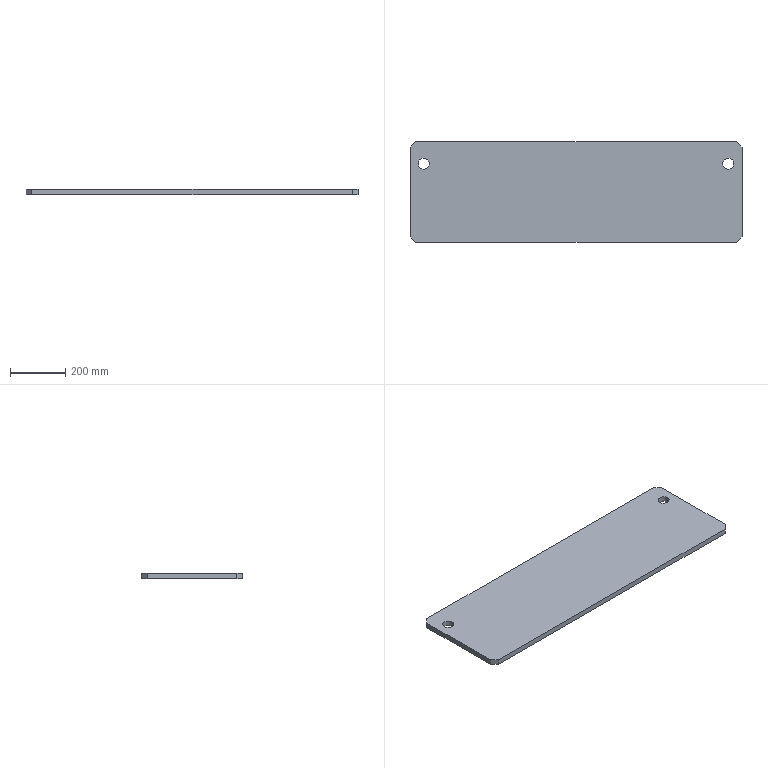Part | SolidWorks | features Chamfer 2, Extrusion 1, ICE 1 | 1 solid | 14 faces | box 1200 x 365 x 20 mm | volume 8693735 mm3 | plane 10 | cylinder 4 | commonest cylinder face diameters 40 x4
STEP:
#1=CARTESIAN_POINT('',(-570.,102.5,0.));
#2=VERTEX_POINT('',#1);
#3=CARTESIAN_POINT('',(-530.,102.5,0.));
#4=VERTEX_POINT('',#3);
#5=CARTESIAN_POINT('',(-550.,102.5,0.));
#6=DIRECTION('',(0.,0.,1.));
#7=DIRECTION('',(1.,0.,0.));
#8=AXIS2_PLACEMENT_3D('',#5,#6,#7);
#9=CIRCLE('',#8,20.);
#10=EDGE_CURVE('',#2,#4,#9,.T.);
#11=ORIENTED_EDGE('',*,*,#10,.F.);
#12=CARTESIAN_POINT('',(-570.,102.5,20.));
#13=VERTEX_POINT('',#12);
#14=CARTESIAN_POINT('',(-570.,102.5,0.));
#15=DIRECTION('',(0.,0.,1.));
#16=VECTOR('',#15,1000.);
#17=LINE('',#14,#16);
#18=EDGE_CURVE('',#2,#13,#17,.T.);
#19=ORIENTED_EDGE('',*,*,#18,.T.);
#20=CARTESIAN_POINT('',(-530.,102.5,20.));
#21=VERTEX_POINT('',#20);
#22=CARTESIAN_POINT('',(-550.,102.5,20.));
#23=DIRECTION('',(0.,0.,1.));
#24=DIRECTION('',(1.,0.,0.));
#25=AXIS2_PLACEMENT_3D('',#22,#23,#24);
#26=CIRCLE('',#25,20.);
#27=EDGE_CURVE('',#13,#21,#26,.T.);
#28=ORIENTED_EDGE('',*,*,#27,.T.);
#29=CARTESIAN_POINT('',(-530.,102.5,0.));
#30=DIRECTION('',(0.,0.,1.));
#31=VECTOR('',#30,1000.);
#32=LINE('',#29,#31);
#33=EDGE_CURVE('',#4,#21,#32,.T.);
#34=ORIENTED_EDGE('',*,*,#33,.F.);
#35=EDGE_LOOP('',(#11,#19,#28,#34));
#36=FACE_OUTER_BOUND('',#35,.T.);
#37=CARTESIAN_POINT('',(-550.,102.5,0.));
#38=DIRECTION('',(0.,0.,1.));
#39=DIRECTION('',(1.,0.,0.));
#40=AXIS2_PLACEMENT_3D('',#37,#38,#39);
#41=CYLINDRICAL_SURFACE('',#40,20.);
#42=ADVANCED_FACE('',(#36),#41,.F.);
#43=CARTESIAN_POINT('',(530.,102.5,0.));
#44=VERTEX_POINT('',#43);
#45=CARTESIAN_POINT('',(570.,102.5,0.));
#46=VERTEX_POINT('',#45);
#47=CARTESIAN_POINT('',(550.,102.5,0.));
#48=DIRECTION('',(0.,0.,1.));
#49=DIRECTION('',(-1.,0.,0.));
#50=AXIS2_PLACEMENT_3D('',#47,#48,#49);
#51=CIRCLE('',#50,20.);
#52=EDGE_CURVE('',#44,#46,#51,.T.);
#53=ORIENTED_EDGE('',*,*,#52,.F.);
#54=CARTESIAN_POINT('',(530.,102.5,20.));
#55=VERTEX_POINT('',#54);
#56=CARTESIAN_POINT('',(530.,102.5,0.));
#57=DIRECTION('',(0.,0.,1.));
#58=VECTOR('',#57,1000.);
#59=LINE('',#56,#58);
#60=EDGE_CURVE('',#44,#55,#59,.T.);
#61=ORIENTED_EDGE('',*,*,#60,.T.);
#62=CARTESIAN_POINT('',(570.,102.5,20.));
#63=VERTEX_POINT('',#62);
#64=CARTESIAN_POINT('',(550.,102.5,20.));
#65=DIRECTION('',(0.,0.,1.));
#66=DIRECTION('',(1.,0.,0.));
#67=AXIS2_PLACEMENT_3D('',#64,#65,#66);
#68=CIRCLE('',#67,20.);
#69=EDGE_CURVE('',#55,#63,#68,.T.);
#70=ORIENTED_EDGE('',*,*,#69,.T.);
#71=CARTESIAN_POINT('',(570.,102.5,0.));
#72=DIRECTION('',(0.,0.,1.));
#73=VECTOR('',#72,1000.);
#74=LINE('',#71,#73);
#75=EDGE_CURVE('',#46,#63,#74,.T.);
#76=ORIENTED_EDGE('',*,*,#75,.F.);
#77=EDGE_LOOP('',(#53,#61,#70,#76));
#78=FACE_OUTER_BOUND('',#77,.T.);
#79=CARTESIAN_POINT('',(550.,102.5,0.));
#80=DIRECTION('',(0.,0.,1.));
#81=DIRECTION('',(1.,0.,0.));
#82=AXIS2_PLACEMENT_3D('',#79,#80,#81);
#83=CYLINDRICAL_SURFACE('',#82,20.);
#84=ADVANCED_FACE('',(#78),#83,.F.);
#85=CARTESIAN_POINT('',(600.,-162.5,20.));
#86=VERTEX_POINT('',#85);
#87=CARTESIAN_POINT('',(600.,162.5,20.));
#88=VERTEX_POINT('',#87);
#89=CARTESIAN_POINT('',(600.,182.5,20.));
#90=DIRECTION('',(0.,1.,0.));
#91=VECTOR('',#90,1000.);
#92=LINE('',#89,#91);
#93=EDGE_CURVE('',#86,#88,#92,.T.);
#94=ORIENTED_EDGE('',*,*,#93,.F.);
#95=CARTESIAN_POINT('',(600.,-162.5,0.));
#96=VERTEX_POINT('',#95);
#97=CARTESIAN_POINT('',(600.,-162.5,20.));
#98=DIRECTION('',(0.,0.,-1.));
#99=VECTOR('',#98,1000.);
#100=LINE('',#97,#99);
#101=EDGE_CURVE('',#86,#96,#100,.T.);
#102=ORIENTED_EDGE('',*,*,#101,.T.);
#103=CARTESIAN_POINT('',(600.,162.5,0.));
#104=VERTEX_POINT('',#103);
#105=CARTESIAN_POINT('',(600.,182.5,0.));
#106=DIRECTION('',(0.,1.,0.));
#107=VECTOR('',#106,1000.);
#108=LINE('',#105,#107);
#109=EDGE_CURVE('',#96,#104,#108,.T.);
#110=ORIENTED_EDGE('',*,*,#109,.T.);
#111=CARTESIAN_POINT('',(600.,162.5,20.));
#112=DIRECTION('',(0.,0.,1.));
#113=VECTOR('',#112,1000.);
#114=LINE('',#111,#113);
#115=EDGE_CURVE('',#104,#88,#114,.T.);
#116=ORIENTED_EDGE('',*,*,#115,.T.);
#117=EDGE_LOOP('',(#94,#102,#110,#116));
#118=FACE_OUTER_BOUND('',#117,.T.);
#119=CARTESIAN_POINT('',(600.,182.5,20.));
#120=DIRECTION('',(-1.,0.,0.));
#121=DIRECTION('',(0.,-1.,0.));
#122=AXIS2_PLACEMENT_3D('',#119,#120,#121);
#123=PLANE('',#122);
#124=ADVANCED_FACE('',(#118),#123,.F.);
#125=CARTESIAN_POINT('',(580.,182.5,20.));
#126=VERTEX_POINT('',#125);
#127=CARTESIAN_POINT('',(-580.,182.5,20.));
#128=VERTEX_POINT('',#127);
#129=CARTESIAN_POINT('',(-600.,182.5,20.));
#130=DIRECTION('',(-1.,0.,0.));
#131=VECTOR('',#130,1000.);
#132=LINE('',#129,#131);
#133=EDGE_CURVE('',#126,#128,#132,.T.);
#134=ORIENTED_EDGE('',*,*,#133,.F.);
#135=CARTESIAN_POINT('',(580.,182.5,0.));
#136=VERTEX_POINT('',#135);
#137=CARTESIAN_POINT('',(580.,182.5,20.));
#138=DIRECTION('',(0.,0.,-1.));
#139=VECTOR('',#138,1000.);
#140=LINE('',#137,#139);
#141=EDGE_CURVE('',#126,#136,#140,.T.);
#142=ORIENTED_EDGE('',*,*,#141,.T.);
#143=CARTESIAN_POINT('',(-580.,182.5,0.));
#144=VERTEX_POINT('',#143);
#145=CARTESIAN_POINT('',(-600.,182.5,0.));
#146=DIRECTION('',(-1.,0.,0.));
#147=VECTOR('',#146,1000.);
#148=LINE('',#145,#147);
#149=EDGE_CURVE('',#136,#144,#148,.T.);
#150=ORIENTED_EDGE('',*,*,#149,.T.);
#151=CARTESIAN_POINT('',(-580.,182.5,20.));
#152=DIRECTION('',(0.,0.,1.));
#153=VECTOR('',#152,1000.);
#154=LINE('',#151,#153);
#155=EDGE_CURVE('',#144,#128,#154,.T.);
#156=ORIENTED_EDGE('',*,*,#155,.T.);
#157=EDGE_LOOP('',(#134,#142,#150,#156));
#158=FACE_OUTER_BOUND('',#157,.T.);
#159=CARTESIAN_POINT('',(-600.,182.5,20.));
#160=DIRECTION('',(0.,-1.,0.));
#161=DIRECTION('',(0.,0.,-1.));
#162=AXIS2_PLACEMENT_3D('',#159,#160,#161);
#163=PLANE('',#162);
#164=ADVANCED_FACE('',(#158),#163,.F.);
#165=CARTESIAN_POINT('',(-600.,162.5,0.));
#166=VERTEX_POINT('',#165);
#167=CARTESIAN_POINT('',(-600.,-162.5,0.));
#168=VERTEX_POINT('',#167);
#169=CARTESIAN_POINT('',(-600.,182.5,0.));
#170=DIRECTION('',(0.,-1.,0.));
#171=VECTOR('',#170,1000.);
#172=LINE('',#169,#171);
#173=EDGE_CURVE('',#166,#168,#172,.T.);
#174=ORIENTED_EDGE('',*,*,#173,.T.);
#175=CARTESIAN_POINT('',(-600.,-162.5,20.));
#176=VERTEX_POINT('',#175);
#177=CARTESIAN_POINT('',(-600.,-162.5,20.));
#178=DIRECTION('',(0.,0.,1.));
#179=VECTOR('',#178,1000.);
#180=LINE('',#177,#179);
#181=EDGE_CURVE('',#168,#176,#180,.T.);
#182=ORIENTED_EDGE('',*,*,#181,.T.);
#183=CARTESIAN_POINT('',(-600.,162.5,20.));
#184=VERTEX_POINT('',#183);
#185=CARTESIAN_POINT('',(-600.,182.5,20.));
#186=DIRECTION('',(0.,-1.,0.));
#187=VECTOR('',#186,1000.);
#188=LINE('',#185,#187);
#189=EDGE_CURVE('',#184,#176,#188,.T.);
#190=ORIENTED_EDGE('',*,*,#189,.F.);
#191=CARTESIAN_POINT('',(-600.,162.5,20.));
#192=DIRECTION('',(0.,0.,-1.));
#193=VECTOR('',#192,1000.);
#194=LINE('',#191,#193);
#195=EDGE_CURVE('',#184,#166,#194,.T.);
#196=ORIENTED_EDGE('',*,*,#195,.T.);
#197=EDGE_LOOP('',(#174,#182,#190,#196));
#198=FACE_OUTER_BOUND('',#197,.T.);
#199=CARTESIAN_POINT('',(-600.,182.5,20.));
#200=DIRECTION('',(1.,0.,0.));
#201=DIRECTION('',(0.,1.,0.));
#202=AXIS2_PLACEMENT_3D('',#199,#200,#201);
#203=PLANE('',#202);
#204=ADVANCED_FACE('',(#198),#203,.F.);
#205=CARTESIAN_POINT('',(-580.,-182.5,20.));
#206=VERTEX_POINT('',#205);
#207=CARTESIAN_POINT('',(580.,-182.5,20.));
#208=VERTEX_POINT('',#207);
#209=CARTESIAN_POINT('',(-600.,-182.5,20.));
#210=DIRECTION('',(1.,0.,0.));
#211=VECTOR('',#210,1000.);
#212=LINE('',#209,#211);
#213=EDGE_CURVE('',#206,#208,#212,.T.);
#214=ORIENTED_EDGE('',*,*,#213,.F.);
#215=CARTESIAN_POINT('',(-580.,-182.5,0.));
#216=VERTEX_POINT('',#215);
#217=CARTESIAN_POINT('',(-580.,-182.5,20.));
#218=DIRECTION('',(0.,0.,-1.));
#219=VECTOR('',#218,1000.);
#220=LINE('',#217,#219);
#221=EDGE_CURVE('',#206,#216,#220,.T.);
#222=ORIENTED_EDGE('',*,*,#221,.T.);
#223=CARTESIAN_POINT('',(580.,-182.5,0.));
#224=VERTEX_POINT('',#223);
#225=CARTESIAN_POINT('',(-600.,-182.5,0.));
#226=DIRECTION('',(1.,0.,0.));
#227=VECTOR('',#226,1000.);
#228=LINE('',#225,#227);
#229=EDGE_CURVE('',#216,#224,#228,.T.);
#230=ORIENTED_EDGE('',*,*,#229,.T.);
#231=CARTESIAN_POINT('',(580.,-182.5,20.));
#232=DIRECTION('',(0.,0.,1.));
#233=VECTOR('',#232,1000.);
#234=LINE('',#231,#233);
#235=EDGE_CURVE('',#224,#208,#234,.T.);
#236=ORIENTED_EDGE('',*,*,#235,.T.);
#237=EDGE_LOOP('',(#214,#222,#230,#236));
#238=FACE_OUTER_BOUND('',#237,.T.);
#239=CARTESIAN_POINT('',(-600.,-182.5,20.));
#240=DIRECTION('',(0.,1.,0.));
#241=DIRECTION('',(0.,0.,1.));
#242=AXIS2_PLACEMENT_3D('',#239,#240,#241);
#243=PLANE('',#242);
#244=ADVANCED_FACE('',(#238),#243,.F.);
#245=CARTESIAN_POINT('',(-550.,102.5,20.));
#246=DIRECTION('',(0.,0.,1.));
#247=DIRECTION('',(1.,0.,0.));
#248=AXIS2_PLACEMENT_3D('',#245,#246,#247);
#249=CIRCLE('',#248,20.);
#250=EDGE_CURVE('',#21,#13,#249,.T.);
#251=ORIENTED_EDGE('',*,*,#250,.F.);
#252=ORIENTED_EDGE('',*,*,#27,.F.);
#253=EDGE_LOOP('',(#251,#252));
#254=FACE_BOUND('',#253,.T.);
#255=CARTESIAN_POINT('',(550.,102.5,20.));
#256=DIRECTION('',(0.,0.,1.));
#257=DIRECTION('',(1.,0.,0.));
#258=AXIS2_PLACEMENT_3D('',#255,#256,#257);
#259=CIRCLE('',#258,20.);
#260=EDGE_CURVE('',#63,#55,#259,.T.);
#261=ORIENTED_EDGE('',*,*,#260,.F.);
#262=ORIENTED_EDGE('',*,*,#69,.F.);
#263=EDGE_LOOP('',(#261,#262));
#264=FACE_BOUND('',#263,.T.);
#265=ORIENTED_EDGE('',*,*,#189,.T.);
#266=CARTESIAN_POINT('',(-381.25,-381.25,20.));
#267=DIRECTION('',(0.7071,-0.7071,0.));
#268=VECTOR('',#267,1000.);
#269=LINE('',#266,#268);
#270=EDGE_CURVE('',#176,#206,#269,.T.);
#271=ORIENTED_EDGE('',*,*,#270,.T.);
#272=ORIENTED_EDGE('',*,*,#213,.T.);
#273=CARTESIAN_POINT('',(381.25,-381.25,20.));
#274=DIRECTION('',(0.7071,0.7071,0.));
#275=VECTOR('',#274,1000.);
#276=LINE('',#273,#275);
#277=EDGE_CURVE('',#208,#86,#276,.T.);
#278=ORIENTED_EDGE('',*,*,#277,.T.);
#279=ORIENTED_EDGE('',*,*,#93,.T.);
#280=CARTESIAN_POINT('',(381.25,381.25,20.));
#281=DIRECTION('',(-0.7071,0.7071,0.));
#282=VECTOR('',#281,1000.);
#283=LINE('',#280,#282);
#284=EDGE_CURVE('',#88,#126,#283,.T.);
#285=ORIENTED_EDGE('',*,*,#284,.T.);
#286=ORIENTED_EDGE('',*,*,#133,.T.);
#287=CARTESIAN_POINT('',(-381.25,381.25,20.));
#288=DIRECTION('',(-0.7071,-0.7071,0.));
#289=VECTOR('',#288,1000.);
#290=LINE('',#287,#289);
#291=EDGE_CURVE('',#128,#184,#290,.T.);
#292=ORIENTED_EDGE('',*,*,#291,.T.);
#293=EDGE_LOOP('',(#265,#271,#272,#278,#279,#285,#286,#292));
#294=FACE_OUTER_BOUND('',#293,.T.);
#295=CARTESIAN_POINT('',(0.,0.,20.));
#296=DIRECTION('',(0.,0.,1.));
#297=DIRECTION('',(1.,0.,0.));
#298=AXIS2_PLACEMENT_3D('',#295,#296,#297);
#299=PLANE('',#298);
#300=ADVANCED_FACE('',(#254,#264,#294),#299,.T.);
#301=CARTESIAN_POINT('',(-550.,102.5,0.));
#302=DIRECTION('',(0.,0.,1.));
#303=DIRECTION('',(1.,0.,0.));
#304=AXIS2_PLACEMENT_3D('',#301,#302,#303);
#305=CIRCLE('',#304,20.);
#306=EDGE_CURVE('',#4,#2,#305,.T.);
#307=ORIENTED_EDGE('',*,*,#306,.T.);
#308=ORIENTED_EDGE('',*,*,#10,.T.);
#309=EDGE_LOOP('',(#307,#308));
#310=FACE_BOUND('',#309,.T.);
#311=CARTESIAN_POINT('',(550.,102.5,0.));
#312=DIRECTION('',(0.,0.,1.));
#313=DIRECTION('',(-1.,0.,0.));
#314=AXIS2_PLACEMENT_3D('',#311,#312,#313);
#315=CIRCLE('',#314,20.);
#316=EDGE_CURVE('',#46,#44,#315,.T.);
#317=ORIENTED_EDGE('',*,*,#316,.T.);
#318=ORIENTED_EDGE('',*,*,#52,.T.);
#319=EDGE_LOOP('',(#317,#318));
#320=FACE_BOUND('',#319,.T.);
#321=ORIENTED_EDGE('',*,*,#229,.F.);
#322=CARTESIAN_POINT('',(-580.,-182.5,0.));
#323=DIRECTION('',(-0.7071,0.7071,0.));
#324=VECTOR('',#323,1000.);
#325=LINE('',#322,#324);
#326=EDGE_CURVE('',#216,#168,#325,.T.);
#327=ORIENTED_EDGE('',*,*,#326,.T.);
#328=ORIENTED_EDGE('',*,*,#173,.F.);
#329=CARTESIAN_POINT('',(-600.,162.5,0.));
#330=DIRECTION('',(0.7071,0.7071,0.));
#331=VECTOR('',#330,1000.);
#332=LINE('',#329,#331);
#333=EDGE_CURVE('',#166,#144,#332,.T.);
#334=ORIENTED_EDGE('',*,*,#333,.T.);
#335=ORIENTED_EDGE('',*,*,#149,.F.);
#336=CARTESIAN_POINT('',(580.,182.5,0.));
#337=DIRECTION('',(0.7071,-0.7071,0.));
#338=VECTOR('',#337,1000.);
#339=LINE('',#336,#338);
#340=EDGE_CURVE('',#136,#104,#339,.T.);
#341=ORIENTED_EDGE('',*,*,#340,.T.);
#342=ORIENTED_EDGE('',*,*,#109,.F.);
#343=CARTESIAN_POINT('',(600.,-162.5,0.));
#344=DIRECTION('',(-0.7071,-0.7071,0.));
#345=VECTOR('',#344,1000.);
#346=LINE('',#343,#345);
#347=EDGE_CURVE('',#96,#224,#346,.T.);
#348=ORIENTED_EDGE('',*,*,#347,.T.);
#349=EDGE_LOOP('',(#321,#327,#328,#334,#335,#341,#342,#348));
#350=FACE_OUTER_BOUND('',#349,.T.);
#351=CARTESIAN_POINT('',(0.,0.,0.));
#352=DIRECTION('',(0.,0.,1.));
#353=DIRECTION('',(1.,0.,0.));
#354=AXIS2_PLACEMENT_3D('',#351,#352,#353);
#355=PLANE('',#354);
#356=ADVANCED_FACE('',(#310,#320,#350),#355,.F.);
#357=ORIENTED_EDGE('',*,*,#60,.F.);
#358=ORIENTED_EDGE('',*,*,#316,.F.);
#359=ORIENTED_EDGE('',*,*,#75,.T.);
#360=ORIENTED_EDGE('',*,*,#260,.T.);
#361=EDGE_LOOP('',(#357,#358,#359,#360));
#362=FACE_OUTER_BOUND('',#361,.T.);
#363=CARTESIAN_POINT('',(550.,102.5,0.));
#364=DIRECTION('',(0.,0.,1.));
#365=DIRECTION('',(1.,0.,0.));
#366=AXIS2_PLACEMENT_3D('',#363,#364,#365);
#367=CYLINDRICAL_SURFACE('',#366,20.);
#368=ADVANCED_FACE('',(#362),#367,.F.);
#369=ORIENTED_EDGE('',*,*,#18,.F.);
#370=ORIENTED_EDGE('',*,*,#306,.F.);
#371=ORIENTED_EDGE('',*,*,#33,.T.);
#372=ORIENTED_EDGE('',*,*,#250,.T.);
#373=EDGE_LOOP('',(#369,#370,#371,#372));
#374=FACE_OUTER_BOUND('',#373,.T.);
#375=CARTESIAN_POINT('',(-550.,102.5,0.));
#376=DIRECTION('',(0.,0.,1.));
#377=DIRECTION('',(1.,0.,0.));
#378=AXIS2_PLACEMENT_3D('',#375,#376,#377);
#379=CYLINDRICAL_SURFACE('',#378,20.);
#380=ADVANCED_FACE('',(#374),#379,.F.);
#381=ORIENTED_EDGE('',*,*,#284,.F.);
#382=ORIENTED_EDGE('',*,*,#115,.F.);
#383=ORIENTED_EDGE('',*,*,#340,.F.);
#384=ORIENTED_EDGE('',*,*,#141,.F.);
#385=EDGE_LOOP('',(#381,#382,#383,#384));
#386=FACE_OUTER_BOUND('',#385,.T.);
#387=CARTESIAN_POINT('',(580.,182.5,20.));
#388=DIRECTION('',(-0.7071,-0.7071,0.));
#389=DIRECTION('',(0.,0.,-1.));
#390=AXIS2_PLACEMENT_3D('',#387,#388,#389);
#391=PLANE('',#390);
#392=ADVANCED_FACE('',(#386),#391,.F.);
#393=ORIENTED_EDGE('',*,*,#291,.F.);
#394=ORIENTED_EDGE('',*,*,#155,.F.);
#395=ORIENTED_EDGE('',*,*,#333,.F.);
#396=ORIENTED_EDGE('',*,*,#195,.F.);
#397=EDGE_LOOP('',(#393,#394,#395,#396));
#398=FACE_OUTER_BOUND('',#397,.T.);
#399=CARTESIAN_POINT('',(-600.,162.5,20.));
#400=DIRECTION('',(0.7071,-0.7071,0.));
#401=DIRECTION('',(0.,0.,-1.));
#402=AXIS2_PLACEMENT_3D('',#399,#400,#401);
#403=PLANE('',#402);
#404=ADVANCED_FACE('',(#398),#403,.F.);
#405=ORIENTED_EDGE('',*,*,#270,.F.);
#406=ORIENTED_EDGE('',*,*,#181,.F.);
#407=ORIENTED_EDGE('',*,*,#326,.F.);
#408=ORIENTED_EDGE('',*,*,#221,.F.);
#409=EDGE_LOOP('',(#405,#406,#407,#408));
#410=FACE_OUTER_BOUND('',#409,.T.);
#411=CARTESIAN_POINT('',(-580.,-182.5,20.));
#412=DIRECTION('',(0.7071,0.7071,0.));
#413=DIRECTION('',(0.,0.,-1.));
#414=AXIS2_PLACEMENT_3D('',#411,#412,#413);
#415=PLANE('',#414);
#416=ADVANCED_FACE('',(#410),#415,.F.);
#417=ORIENTED_EDGE('',*,*,#277,.F.);
#418=ORIENTED_EDGE('',*,*,#235,.F.);
#419=ORIENTED_EDGE('',*,*,#347,.F.);
#420=ORIENTED_EDGE('',*,*,#101,.F.);
#421=EDGE_LOOP('',(#417,#418,#419,#420));
#422=FACE_OUTER_BOUND('',#421,.T.);
#423=CARTESIAN_POINT('',(600.,-162.5,20.));
#424=DIRECTION('',(-0.7071,0.7071,0.));
#425=DIRECTION('',(0.,0.,-1.));
#426=AXIS2_PLACEMENT_3D('',#423,#424,#425);
#427=PLANE('',#426);
#428=ADVANCED_FACE('',(#422),#427,.F.);
#429=CLOSED_SHELL('',(#42,#84,#124,#164,#204,#244,#300,#356,#368,#380,#392,#404,#416,#428));
#430=MANIFOLD_SOLID_BREP('',#429);
#431=CARTESIAN_POINT('',(0.,0.,0.));
#432=DIRECTION('',(0.,0.,1.));
#433=DIRECTION('',(1.,0.,0.));
#434=AXIS2_PLACEMENT_3D('',#431,#432,#433);
#435=(LENGTH_UNIT()NAMED_UNIT(*)SI_UNIT(.MILLI.,.METRE.));
#436=UNCERTAINTY_MEASURE_WITH_UNIT(LENGTH_MEASURE(0.00001),#435,'','');
#437=(NAMED_UNIT(*)PLANE_ANGLE_UNIT()SI_UNIT($,.RADIAN.));
#438=(NAMED_UNIT(*)SI_UNIT($,.STERADIAN.)SOLID_ANGLE_UNIT());
#439=(GEOMETRIC_REPRESENTATION_CONTEXT(3)GLOBAL_UNCERTAINTY_ASSIGNED_CONTEXT((#436))GLOBAL_UNIT_ASSIGNED_CONTEXT((#435,#437,#438))REPRESENTATION_CONTEXT('',''));
#440=ADVANCED_BREP_SHAPE_REPRESENTATION('',(#430,#434),#439);